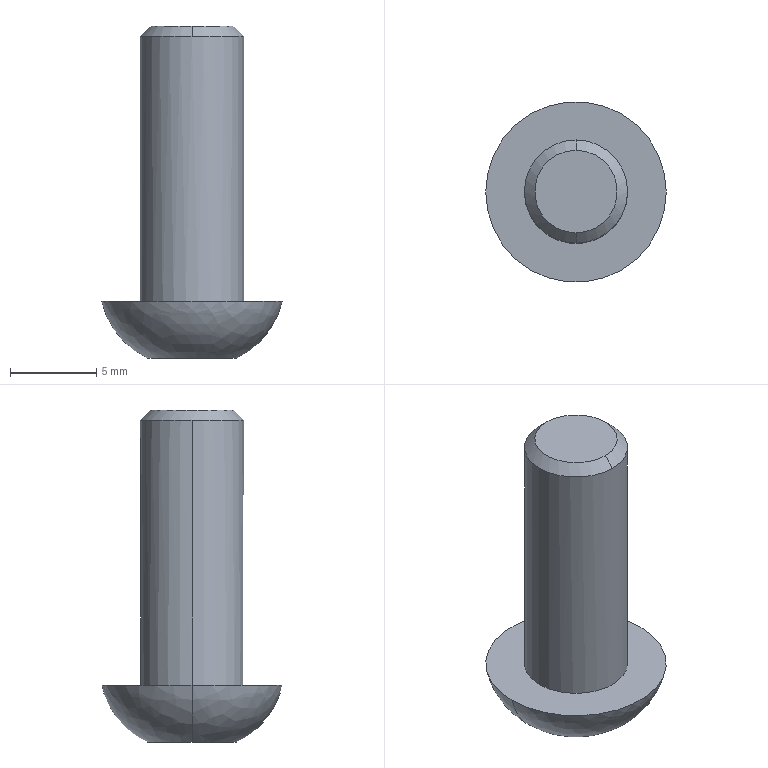Part | STEP file | LE-BYS-M6X16_PN_0013 | 1 solid | 23 faces | box 10.5 x 10.5 x 19.3 mm | volume 623.238 mm3 | plane 15 | cone 4 | spline 2 | cylinder 2 | commonest cylinder face diameters 6 x2
STEP:
#1=CARTESIAN_POINT('',(-2.6,0.,-3.3));
#2=VERTEX_POINT('',#1);
#3=CARTESIAN_POINT('',(2.6,0.,-3.3));
#4=VERTEX_POINT('',#3);
#5=CARTESIAN_POINT('',(0.,0.,-3.3));
#6=DIRECTION('',(0.,0.,1.));
#7=DIRECTION('',(-1.,0.,0.));
#8=AXIS2_PLACEMENT_3D('',#5,#6,#7);
#9=CIRCLE('',#8,2.6);
#10=EDGE_CURVE('',#2,#4,#9,.T.);
#11=ORIENTED_EDGE('',*,*,#10,.T.);
#12=CARTESIAN_POINT('',(5.25,0.,0.));
#13=VERTEX_POINT('',#12);
#14=CARTESIAN_POINT('',(0.5657,0.,1.048));
#15=DIRECTION('',(0.,-1.,0.));
#16=DIRECTION('',(1.,0.,0.));
#17=AXIS2_PLACEMENT_3D('',#14,#15,#16);
#18=CIRCLE('',#17,4.8);
#19=EDGE_CURVE('',#4,#13,#18,.T.);
#20=ORIENTED_EDGE('',*,*,#19,.T.);
#21=CARTESIAN_POINT('',(-5.25,0.,0.));
#22=VERTEX_POINT('',#21);
#23=CARTESIAN_POINT('',(0.,0.,0.));
#24=DIRECTION('',(0.,0.,1.));
#25=DIRECTION('',(-1.,0.,0.));
#26=AXIS2_PLACEMENT_3D('',#23,#24,#25);
#27=CIRCLE('',#26,5.25);
#28=EDGE_CURVE('',#22,#13,#27,.T.);
#29=ORIENTED_EDGE('',*,*,#28,.F.);
#30=CARTESIAN_POINT('',(-0.5657,0.,1.048));
#31=DIRECTION('',(0.,1.,0.));
#32=DIRECTION('',(-1.,0.,0.));
#33=AXIS2_PLACEMENT_3D('',#30,#31,#32);
#34=CIRCLE('',#33,4.8);
#35=EDGE_CURVE('',#2,#22,#34,.T.);
#36=ORIENTED_EDGE('',*,*,#35,.F.);
#37=EDGE_LOOP('',(#11,#20,#29,#36));
#38=FACE_OUTER_BOUND('',#37,.T.);
#39=CARTESIAN_POINT('',(2.6,0.,-3.3));
#40=CARTESIAN_POINT('',(2.6,-5.2,-3.3));
#41=CARTESIAN_POINT('',(-2.6,-5.2,-3.3));
#42=CARTESIAN_POINT('',(-2.6,0.,-3.3));
#43=CARTESIAN_POINT('',(3.971,0.,-2.658));
#44=CARTESIAN_POINT('',(3.971,-7.943,-2.658));
#45=CARTESIAN_POINT('',(-3.971,-7.943,-2.658));
#46=CARTESIAN_POINT('',(-3.971,0.,-2.658));
#47=CARTESIAN_POINT('',(4.92,0.,-1.478));
#48=CARTESIAN_POINT('',(4.92,-9.839,-1.478));
#49=CARTESIAN_POINT('',(-4.92,-9.839,-1.478));
#50=CARTESIAN_POINT('',(-4.92,0.,-1.478));
#51=CARTESIAN_POINT('',(5.25,0.,0.));
#52=CARTESIAN_POINT('',(5.25,-10.5,0.));
#53=CARTESIAN_POINT('',(-5.25,-10.5,0.));
#54=CARTESIAN_POINT('',(-5.25,0.,0.));
#55=(BOUNDED_SURFACE()B_SPLINE_SURFACE(3,3,((#39,#40,#41,#42),(#43,#44,#45,#46),(#47,#48,#49,#50),(#51,#52,#53,#54)),.UNSPECIFIED.,.F.,.F.,.T.)B_SPLINE_SURFACE_WITH_KNOTS((4,4),(4,4),(0.,1.),(0.,1.),.UNSPECIFIED.)GEOMETRIC_REPRESENTATION_ITEM()RATIONAL_B_SPLINE_SURFACE(((1.,0.3333,0.3333,1.),(0.9317,0.3106,0.3106,0.9317),(0.9317,0.3106,0.3106,0.9317),(1.,0.3333,0.3333,1.)))REPRESENTATION_ITEM('')SURFACE());
#56=ADVANCED_FACE('',(#38),#55,.T.);
#57=CARTESIAN_POINT('',(0.,3.,15.4));
#58=VERTEX_POINT('',#57);
#59=CARTESIAN_POINT('',(3.,0.,15.4));
#60=VERTEX_POINT('',#59);
#61=CARTESIAN_POINT('',(0.,0.,15.4));
#62=DIRECTION('',(0.,0.,-1.));
#63=DIRECTION('',(-1.,0.,0.));
#64=AXIS2_PLACEMENT_3D('',#61,#62,#63);
#65=CIRCLE('',#64,3.);
#66=EDGE_CURVE('',#58,#60,#65,.T.);
#67=ORIENTED_EDGE('',*,*,#66,.T.);
#68=CARTESIAN_POINT('',(3.,0.,0.));
#69=VERTEX_POINT('',#68);
#70=CARTESIAN_POINT('',(3.,0.,16.));
#71=DIRECTION('',(0.,0.,-1.));
#72=VECTOR('',#71,1000.);
#73=LINE('',#70,#72);
#74=EDGE_CURVE('',#60,#69,#73,.T.);
#75=ORIENTED_EDGE('',*,*,#74,.T.);
#76=CARTESIAN_POINT('',(-3.,0.,0.));
#77=VERTEX_POINT('',#76);
#78=CARTESIAN_POINT('',(0.,0.,0.));
#79=DIRECTION('',(0.,0.,1.));
#80=DIRECTION('',(-1.,0.,0.));
#81=AXIS2_PLACEMENT_3D('',#78,#79,#80);
#82=CIRCLE('',#81,3.);
#83=EDGE_CURVE('',#69,#77,#82,.T.);
#84=ORIENTED_EDGE('',*,*,#83,.T.);
#85=CARTESIAN_POINT('',(-3.,0.,15.4));
#86=VERTEX_POINT('',#85);
#87=CARTESIAN_POINT('',(-3.,0.,16.));
#88=DIRECTION('',(0.,0.,-1.));
#89=VECTOR('',#88,1000.);
#90=LINE('',#87,#89);
#91=EDGE_CURVE('',#86,#77,#90,.T.);
#92=ORIENTED_EDGE('',*,*,#91,.F.);
#93=CARTESIAN_POINT('',(0.,0.,15.4));
#94=DIRECTION('',(0.,0.,-1.));
#95=DIRECTION('',(-1.,0.,0.));
#96=AXIS2_PLACEMENT_3D('',#93,#94,#95);
#97=CIRCLE('',#96,3.);
#98=EDGE_CURVE('',#86,#58,#97,.T.);
#99=ORIENTED_EDGE('',*,*,#98,.T.);
#100=EDGE_LOOP('',(#67,#75,#84,#92,#99));
#101=FACE_OUTER_BOUND('',#100,.T.);
#102=CARTESIAN_POINT('',(0.,0.,16.));
#103=DIRECTION('',(0.,0.,-1.));
#104=DIRECTION('',(-1.,0.,0.));
#105=AXIS2_PLACEMENT_3D('',#102,#103,#104);
#106=CYLINDRICAL_SURFACE('',#105,3.);
#107=ADVANCED_FACE('',(#101),#106,.T.);
#108=CARTESIAN_POINT('',(0.,2.4,16.));
#109=VERTEX_POINT('',#108);
#110=CARTESIAN_POINT('',(0.,-2.4,16.));
#111=VERTEX_POINT('',#110);
#112=CARTESIAN_POINT('',(0.,0.,16.));
#113=DIRECTION('',(0.,0.,-1.));
#114=DIRECTION('',(0.,1.,0.));
#115=AXIS2_PLACEMENT_3D('',#112,#113,#114);
#116=CIRCLE('',#115,2.4);
#117=EDGE_CURVE('',#109,#111,#116,.T.);
#118=ORIENTED_EDGE('',*,*,#117,.T.);
#119=CARTESIAN_POINT('',(0.,-3.,15.4));
#120=VERTEX_POINT('',#119);
#121=CARTESIAN_POINT('',(0.,-3.,15.4));
#122=DIRECTION('',(0.,-0.7071,-0.7071));
#123=VECTOR('',#122,1000.);
#124=LINE('',#121,#123);
#125=EDGE_CURVE('',#111,#120,#124,.T.);
#126=ORIENTED_EDGE('',*,*,#125,.T.);
#127=CARTESIAN_POINT('',(0.,0.,15.4));
#128=DIRECTION('',(0.,0.,-1.));
#129=DIRECTION('',(-1.,0.,0.));
#130=AXIS2_PLACEMENT_3D('',#127,#128,#129);
#131=CIRCLE('',#130,3.);
#132=EDGE_CURVE('',#60,#120,#131,.T.);
#133=ORIENTED_EDGE('',*,*,#132,.F.);
#134=ORIENTED_EDGE('',*,*,#66,.F.);
#135=CARTESIAN_POINT('',(0.,3.,15.4));
#136=DIRECTION('',(0.,0.7071,-0.7071));
#137=VECTOR('',#136,1000.);
#138=LINE('',#135,#137);
#139=EDGE_CURVE('',#109,#58,#138,.T.);
#140=ORIENTED_EDGE('',*,*,#139,.F.);
#141=EDGE_LOOP('',(#118,#126,#133,#134,#140));
#142=FACE_OUTER_BOUND('',#141,.T.);
#143=CARTESIAN_POINT('',(0.,0.,15.4));
#144=DIRECTION('',(0.,0.,-1.));
#145=DIRECTION('',(0.,1.,0.));
#146=AXIS2_PLACEMENT_3D('',#143,#144,#145);
#147=CONICAL_SURFACE('',#146,3.,0.7854);
#148=ADVANCED_FACE('',(#142),#147,.T.);
#149=CARTESIAN_POINT('',(0.,0.,-0.4953));
#150=VERTEX_POINT('',#149);
#151=CARTESIAN_POINT('',(0.,2.,-1.65));
#152=VERTEX_POINT('',#151);
#153=CARTESIAN_POINT('',(0.,2.,-1.65));
#154=DIRECTION('',(0.,0.866,-0.5));
#155=VECTOR('',#154,1000.);
#156=LINE('',#153,#155);
#157=EDGE_CURVE('',#150,#152,#156,.T.);
#158=ORIENTED_EDGE('',*,*,#157,.F.);
#159=CARTESIAN_POINT('',(0.,-2.,-1.65));
#160=VERTEX_POINT('',#159);
#161=CARTESIAN_POINT('',(0.,-2.,-1.65));
#162=DIRECTION('',(0.,-0.866,-0.5));
#163=VECTOR('',#162,1000.);
#164=LINE('',#161,#163);
#165=EDGE_CURVE('',#150,#160,#164,.T.);
#166=ORIENTED_EDGE('',*,*,#165,.T.);
#167=CARTESIAN_POINT('',(-1.732,-1.,-1.65));
#168=VERTEX_POINT('',#167);
#169=CARTESIAN_POINT('',(0.,0.,-1.65));
#170=DIRECTION('',(0.,0.,1.));
#171=DIRECTION('',(0.,1.,0.));
#172=AXIS2_PLACEMENT_3D('',#169,#170,#171);
#173=CIRCLE('',#172,2.);
#174=EDGE_CURVE('',#168,#160,#173,.T.);
#175=ORIENTED_EDGE('',*,*,#174,.F.);
#176=CARTESIAN_POINT('',(-1.732,1.,-1.65));
#177=VERTEX_POINT('',#176);
#178=CARTESIAN_POINT('',(0.,0.,-1.65));
#179=DIRECTION('',(0.,0.,-1.));
#180=DIRECTION('',(0.,1.,0.));
#181=AXIS2_PLACEMENT_3D('',#178,#179,#180);
#182=CIRCLE('',#181,2.);
#183=EDGE_CURVE('',#168,#177,#182,.T.);
#184=ORIENTED_EDGE('',*,*,#183,.T.);
#185=CARTESIAN_POINT('',(0.,0.,-1.65));
#186=DIRECTION('',(0.,0.,1.));
#187=DIRECTION('',(0.,1.,0.));
#188=AXIS2_PLACEMENT_3D('',#185,#186,#187);
#189=CIRCLE('',#188,2.);
#190=EDGE_CURVE('',#152,#177,#189,.T.);
#191=ORIENTED_EDGE('',*,*,#190,.F.);
#192=EDGE_LOOP('',(#158,#166,#175,#184,#191));
#193=FACE_OUTER_BOUND('',#192,.T.);
#194=CARTESIAN_POINT('',(0.,0.,-1.65));
#195=DIRECTION('',(0.,0.,-1.));
#196=DIRECTION('',(0.,1.,0.));
#197=AXIS2_PLACEMENT_3D('',#194,#195,#196);
#198=CONICAL_SURFACE('',#197,2.,1.047);
#199=ADVANCED_FACE('',(#193),#198,.F.);
#200=ORIENTED_EDGE('',*,*,#74,.F.);
#201=ORIENTED_EDGE('',*,*,#132,.T.);
#202=CARTESIAN_POINT('',(0.,0.,15.4));
#203=DIRECTION('',(0.,0.,-1.));
#204=DIRECTION('',(-1.,0.,0.));
#205=AXIS2_PLACEMENT_3D('',#202,#203,#204);
#206=CIRCLE('',#205,3.);
#207=EDGE_CURVE('',#120,#86,#206,.T.);
#208=ORIENTED_EDGE('',*,*,#207,.T.);
#209=ORIENTED_EDGE('',*,*,#91,.T.);
#210=CARTESIAN_POINT('',(0.,0.,0.));
#211=DIRECTION('',(0.,0.,1.));
#212=DIRECTION('',(-1.,0.,0.));
#213=AXIS2_PLACEMENT_3D('',#210,#211,#212);
#214=CIRCLE('',#213,3.);
#215=EDGE_CURVE('',#77,#69,#214,.T.);
#216=ORIENTED_EDGE('',*,*,#215,.T.);
#217=EDGE_LOOP('',(#200,#201,#208,#209,#216));
#218=FACE_OUTER_BOUND('',#217,.T.);
#219=CARTESIAN_POINT('',(0.,0.,16.));
#220=DIRECTION('',(0.,0.,-1.));
#221=DIRECTION('',(-1.,0.,0.));
#222=AXIS2_PLACEMENT_3D('',#219,#220,#221);
#223=CYLINDRICAL_SURFACE('',#222,3.);
#224=ADVANCED_FACE('',(#218),#223,.T.);
#225=ORIENTED_EDGE('',*,*,#28,.T.);
#226=CARTESIAN_POINT('',(0.,0.,0.));
#227=DIRECTION('',(0.,0.,1.));
#228=DIRECTION('',(-1.,0.,0.));
#229=AXIS2_PLACEMENT_3D('',#226,#227,#228);
#230=CIRCLE('',#229,5.25);
#231=EDGE_CURVE('',#13,#22,#230,.T.);
#232=ORIENTED_EDGE('',*,*,#231,.T.);
#233=EDGE_LOOP('',(#225,#232));
#234=FACE_OUTER_BOUND('',#233,.T.);
#235=ORIENTED_EDGE('',*,*,#215,.F.);
#236=ORIENTED_EDGE('',*,*,#83,.F.);
#237=EDGE_LOOP('',(#235,#236));
#238=FACE_BOUND('',#237,.T.);
#239=CARTESIAN_POINT('',(0.,0.,0.));
#240=DIRECTION('',(0.,0.,1.));
#241=DIRECTION('',(1.,0.,0.));
#242=AXIS2_PLACEMENT_3D('',#239,#240,#241);
#243=PLANE('',#242);
#244=ADVANCED_FACE('',(#234,#238),#243,.T.);
#245=ORIENTED_EDGE('',*,*,#125,.F.);
#246=CARTESIAN_POINT('',(0.,0.,16.));
#247=DIRECTION('',(0.,0.,-1.));
#248=DIRECTION('',(0.,1.,0.));
#249=AXIS2_PLACEMENT_3D('',#246,#247,#248);
#250=CIRCLE('',#249,2.4);
#251=EDGE_CURVE('',#111,#109,#250,.T.);
#252=ORIENTED_EDGE('',*,*,#251,.T.);
#253=ORIENTED_EDGE('',*,*,#139,.T.);
#254=ORIENTED_EDGE('',*,*,#98,.F.);
#255=ORIENTED_EDGE('',*,*,#207,.F.);
#256=EDGE_LOOP('',(#245,#252,#253,#254,#255));
#257=FACE_OUTER_BOUND('',#256,.T.);
#258=CARTESIAN_POINT('',(0.,0.,15.4));
#259=DIRECTION('',(0.,0.,-1.));
#260=DIRECTION('',(0.,1.,0.));
#261=AXIS2_PLACEMENT_3D('',#258,#259,#260);
#262=CONICAL_SURFACE('',#261,3.,0.7854);
#263=ADVANCED_FACE('',(#257),#262,.T.);
#264=ORIENTED_EDGE('',*,*,#19,.F.);
#265=CARTESIAN_POINT('',(0.,0.,-3.3));
#266=DIRECTION('',(0.,0.,1.));
#267=DIRECTION('',(-1.,0.,0.));
#268=AXIS2_PLACEMENT_3D('',#265,#266,#267);
#269=CIRCLE('',#268,2.6);
#270=EDGE_CURVE('',#4,#2,#269,.T.);
#271=ORIENTED_EDGE('',*,*,#270,.T.);
#272=ORIENTED_EDGE('',*,*,#35,.T.);
#273=ORIENTED_EDGE('',*,*,#231,.F.);
#274=EDGE_LOOP('',(#264,#271,#272,#273));
#275=FACE_OUTER_BOUND('',#274,.T.);
#276=CARTESIAN_POINT('',(-2.6,0.,-3.3));
#277=CARTESIAN_POINT('',(-2.6,5.2,-3.3));
#278=CARTESIAN_POINT('',(2.6,5.2,-3.3));
#279=CARTESIAN_POINT('',(2.6,0.,-3.3));
#280=CARTESIAN_POINT('',(-3.971,0.,-2.658));
#281=CARTESIAN_POINT('',(-3.971,7.943,-2.658));
#282=CARTESIAN_POINT('',(3.971,7.943,-2.658));
#283=CARTESIAN_POINT('',(3.971,0.,-2.658));
#284=CARTESIAN_POINT('',(-4.92,0.,-1.478));
#285=CARTESIAN_POINT('',(-4.92,9.839,-1.478));
#286=CARTESIAN_POINT('',(4.92,9.839,-1.478));
#287=CARTESIAN_POINT('',(4.92,0.,-1.478));
#288=CARTESIAN_POINT('',(-5.25,0.,0.));
#289=CARTESIAN_POINT('',(-5.25,10.5,0.));
#290=CARTESIAN_POINT('',(5.25,10.5,0.));
#291=CARTESIAN_POINT('',(5.25,0.,0.));
#292=(BOUNDED_SURFACE()B_SPLINE_SURFACE(3,3,((#276,#277,#278,#279),(#280,#281,#282,#283),(#284,#285,#286,#287),(#288,#289,#290,#291)),.UNSPECIFIED.,.F.,.F.,.F.)B_SPLINE_SURFACE_WITH_KNOTS((4,4),(4,4),(0.,1.),(0.,1.),.UNSPECIFIED.)GEOMETRIC_REPRESENTATION_ITEM()RATIONAL_B_SPLINE_SURFACE(((1.,0.3333,0.3333,1.),(0.9317,0.3106,0.3106,0.9317),(0.9317,0.3106,0.3106,0.9317),(1.,0.3333,0.3333,1.)))REPRESENTATION_ITEM('')SURFACE());
#293=ADVANCED_FACE('',(#275),#292,.T.);
#294=ORIENTED_EDGE('',*,*,#117,.F.);
#295=ORIENTED_EDGE('',*,*,#251,.F.);
#296=EDGE_LOOP('',(#294,#295));
#297=FACE_OUTER_BOUND('',#296,.T.);
#298=CARTESIAN_POINT('',(0.,0.,16.));
#299=DIRECTION('',(0.,0.,-1.));
#300=DIRECTION('',(-1.,0.,0.));
#301=AXIS2_PLACEMENT_3D('',#298,#299,#300);
#302=PLANE('',#301);
#303=ADVANCED_FACE('',(#297),#302,.F.);
#304=CARTESIAN_POINT('',(-1.155,2.,-3.3));
#305=VERTEX_POINT('',#304);
#306=CARTESIAN_POINT('',(1.155,2.,-3.3));
#307=VERTEX_POINT('',#306);
#308=CARTESIAN_POINT('',(0.,2.,-3.3));
#309=DIRECTION('',(1.,0.,0.));
#310=VECTOR('',#309,1000.);
#311=LINE('',#308,#310);
#312=EDGE_CURVE('',#305,#307,#311,.T.);
#313=ORIENTED_EDGE('',*,*,#312,.F.);
#314=CARTESIAN_POINT('',(-2.309,0.,-3.3));
#315=VERTEX_POINT('',#314);
#316=CARTESIAN_POINT('',(-2.309,0.,-3.3));
#317=DIRECTION('',(0.5,0.866,0.));
#318=VECTOR('',#317,1000.);
#319=LINE('',#316,#318);
#320=EDGE_CURVE('',#315,#305,#319,.T.);
#321=ORIENTED_EDGE('',*,*,#320,.F.);
#322=CARTESIAN_POINT('',(-1.155,-2.,-3.3));
#323=VERTEX_POINT('',#322);
#324=CARTESIAN_POINT('',(-1.155,-2.,-3.3));
#325=DIRECTION('',(-0.5,0.866,0.));
#326=VECTOR('',#325,1000.);
#327=LINE('',#324,#326);
#328=EDGE_CURVE('',#323,#315,#327,.T.);
#329=ORIENTED_EDGE('',*,*,#328,.F.);
#330=CARTESIAN_POINT('',(1.155,-2.,-3.3));
#331=VERTEX_POINT('',#330);
#332=CARTESIAN_POINT('',(0.,-2.,-3.3));
#333=DIRECTION('',(-1.,0.,0.));
#334=VECTOR('',#333,1000.);
#335=LINE('',#332,#334);
#336=EDGE_CURVE('',#331,#323,#335,.T.);
#337=ORIENTED_EDGE('',*,*,#336,.F.);
#338=CARTESIAN_POINT('',(2.309,0.,-3.3));
#339=VERTEX_POINT('',#338);
#340=CARTESIAN_POINT('',(2.309,0.,-3.3));
#341=DIRECTION('',(-0.5,-0.866,0.));
#342=VECTOR('',#341,1000.);
#343=LINE('',#340,#342);
#344=EDGE_CURVE('',#339,#331,#343,.T.);
#345=ORIENTED_EDGE('',*,*,#344,.F.);
#346=CARTESIAN_POINT('',(1.155,2.,-3.3));
#347=DIRECTION('',(0.5,-0.866,0.));
#348=VECTOR('',#347,1000.);
#349=LINE('',#346,#348);
#350=EDGE_CURVE('',#307,#339,#349,.T.);
#351=ORIENTED_EDGE('',*,*,#350,.F.);
#352=EDGE_LOOP('',(#313,#321,#329,#337,#345,#351));
#353=FACE_BOUND('',#352,.T.);
#354=ORIENTED_EDGE('',*,*,#10,.F.);
#355=ORIENTED_EDGE('',*,*,#270,.F.);
#356=EDGE_LOOP('',(#354,#355));
#357=FACE_OUTER_BOUND('',#356,.T.);
#358=CARTESIAN_POINT('',(0.,0.,-3.3));
#359=DIRECTION('',(0.,0.,1.));
#360=DIRECTION('',(1.,0.,0.));
#361=AXIS2_PLACEMENT_3D('',#358,#359,#360);
#362=PLANE('',#361);
#363=ADVANCED_FACE('',(#353,#357),#362,.F.);
#364=CARTESIAN_POINT('',(1.732,1.,-1.65));
#365=VERTEX_POINT('',#364);
#366=CARTESIAN_POINT('',(1.155,2.,-1.65));
#367=VERTEX_POINT('',#366);
#368=CARTESIAN_POINT('',(2.309,0.,-1.65));
#369=DIRECTION('',(-0.5,0.866,0.));
#370=VECTOR('',#369,1000.);
#371=LINE('',#368,#370);
#372=EDGE_CURVE('',#365,#367,#371,.T.);
#373=ORIENTED_EDGE('',*,*,#372,.T.);
#374=CARTESIAN_POINT('',(1.155,2.,-1.65));
#375=DIRECTION('',(0.,0.,-1.));
#376=VECTOR('',#375,1000.);
#377=LINE('',#374,#376);
#378=EDGE_CURVE('',#367,#307,#377,.T.);
#379=ORIENTED_EDGE('',*,*,#378,.T.);
#380=ORIENTED_EDGE('',*,*,#350,.T.);
#381=CARTESIAN_POINT('',(2.309,0.,-1.65));
#382=VERTEX_POINT('',#381);
#383=CARTESIAN_POINT('',(2.309,0.,-1.65));
#384=DIRECTION('',(0.,0.,1.));
#385=VECTOR('',#384,1000.);
#386=LINE('',#383,#385);
#387=EDGE_CURVE('',#339,#382,#386,.T.);
#388=ORIENTED_EDGE('',*,*,#387,.T.);
#389=CARTESIAN_POINT('',(2.309,0.,-1.65));
#390=DIRECTION('',(-0.5,0.866,0.));
#391=VECTOR('',#390,1000.);
#392=LINE('',#389,#391);
#393=EDGE_CURVE('',#382,#365,#392,.T.);
#394=ORIENTED_EDGE('',*,*,#393,.T.);
#395=EDGE_LOOP('',(#373,#379,#380,#388,#394));
#396=FACE_OUTER_BOUND('',#395,.T.);
#397=CARTESIAN_POINT('',(2.309,0.,-1.65));
#398=DIRECTION('',(-0.866,-0.5,0.));
#399=DIRECTION('',(0.5,-0.866,0.));
#400=AXIS2_PLACEMENT_3D('',#397,#398,#399);
#401=PLANE('',#400);
#402=ADVANCED_FACE('',(#396),#401,.T.);
#403=CARTESIAN_POINT('',(-1.155,2.,-1.65));
#404=VERTEX_POINT('',#403);
#405=CARTESIAN_POINT('',(0.,2.,-1.65));
#406=DIRECTION('',(-1.,0.,0.));
#407=VECTOR('',#406,1000.);
#408=LINE('',#405,#407);
#409=EDGE_CURVE('',#152,#404,#408,.T.);
#410=ORIENTED_EDGE('',*,*,#409,.T.);
#411=CARTESIAN_POINT('',(-1.155,2.,-1.65));
#412=DIRECTION('',(0.,0.,-1.));
#413=VECTOR('',#412,1000.);
#414=LINE('',#411,#413);
#415=EDGE_CURVE('',#404,#305,#414,.T.);
#416=ORIENTED_EDGE('',*,*,#415,.T.);
#417=ORIENTED_EDGE('',*,*,#312,.T.);
#418=ORIENTED_EDGE('',*,*,#378,.F.);
#419=CARTESIAN_POINT('',(1.155,2.,-1.65));
#420=DIRECTION('',(-1.,0.,0.));
#421=VECTOR('',#420,1000.);
#422=LINE('',#419,#421);
#423=EDGE_CURVE('',#367,#152,#422,.T.);
#424=ORIENTED_EDGE('',*,*,#423,.T.);
#425=EDGE_LOOP('',(#410,#416,#417,#418,#424));
#426=FACE_OUTER_BOUND('',#425,.T.);
#427=CARTESIAN_POINT('',(1.155,2.,-1.65));
#428=DIRECTION('',(0.,-1.,0.));
#429=DIRECTION('',(0.,0.,-1.));
#430=AXIS2_PLACEMENT_3D('',#427,#428,#429);
#431=PLANE('',#430);
#432=ADVANCED_FACE('',(#426),#431,.T.);
#433=CARTESIAN_POINT('',(-2.309,0.,-1.65));
#434=VERTEX_POINT('',#433);
#435=CARTESIAN_POINT('',(-1.155,2.,-1.65));
#436=DIRECTION('',(-0.5,-0.866,0.));
#437=VECTOR('',#436,1000.);
#438=LINE('',#435,#437);
#439=EDGE_CURVE('',#177,#434,#438,.T.);
#440=ORIENTED_EDGE('',*,*,#439,.T.);
#441=CARTESIAN_POINT('',(-2.309,0.,-1.65));
#442=DIRECTION('',(0.,0.,-1.));
#443=VECTOR('',#442,1000.);
#444=LINE('',#441,#443);
#445=EDGE_CURVE('',#434,#315,#444,.T.);
#446=ORIENTED_EDGE('',*,*,#445,.T.);
#447=ORIENTED_EDGE('',*,*,#320,.T.);
#448=ORIENTED_EDGE('',*,*,#415,.F.);
#449=CARTESIAN_POINT('',(-1.155,2.,-1.65));
#450=DIRECTION('',(-0.5,-0.866,0.));
#451=VECTOR('',#450,1000.);
#452=LINE('',#449,#451);
#453=EDGE_CURVE('',#404,#177,#452,.T.);
#454=ORIENTED_EDGE('',*,*,#453,.T.);
#455=EDGE_LOOP('',(#440,#446,#447,#448,#454));
#456=FACE_OUTER_BOUND('',#455,.T.);
#457=CARTESIAN_POINT('',(-1.155,2.,-1.65));
#458=DIRECTION('',(0.866,-0.5,0.));
#459=DIRECTION('',(0.5,0.866,0.));
#460=AXIS2_PLACEMENT_3D('',#457,#458,#459);
#461=PLANE('',#460);
#462=ADVANCED_FACE('',(#456),#461,.T.);
#463=CARTESIAN_POINT('',(-1.155,-2.,-1.65));
#464=VERTEX_POINT('',#463);
#465=CARTESIAN_POINT('',(-1.732,-1.,-1.65));
#466=DIRECTION('',(0.5,-0.866,0.));
#467=VECTOR('',#466,1000.);
#468=LINE('',#465,#467);
#469=EDGE_CURVE('',#168,#464,#468,.T.);
#470=ORIENTED_EDGE('',*,*,#469,.T.);
#471=CARTESIAN_POINT('',(-1.155,-2.,-1.65));
#472=DIRECTION('',(0.,0.,-1.));
#473=VECTOR('',#472,1000.);
#474=LINE('',#471,#473);
#475=EDGE_CURVE('',#464,#323,#474,.T.);
#476=ORIENTED_EDGE('',*,*,#475,.T.);
#477=ORIENTED_EDGE('',*,*,#328,.T.);
#478=ORIENTED_EDGE('',*,*,#445,.F.);
#479=CARTESIAN_POINT('',(-2.309,0.,-1.65));
#480=DIRECTION('',(0.5,-0.866,0.));
#481=VECTOR('',#480,1000.);
#482=LINE('',#479,#481);
#483=EDGE_CURVE('',#434,#168,#482,.T.);
#484=ORIENTED_EDGE('',*,*,#483,.T.);
#485=EDGE_LOOP('',(#470,#476,#477,#478,#484));
#486=FACE_OUTER_BOUND('',#485,.T.);
#487=CARTESIAN_POINT('',(-2.309,0.,-1.65));
#488=DIRECTION('',(0.866,0.5,0.));
#489=DIRECTION('',(-0.5,0.866,0.));
#490=AXIS2_PLACEMENT_3D('',#487,#488,#489);
#491=PLANE('',#490);
#492=ADVANCED_FACE('',(#486),#491,.T.);
#493=CARTESIAN_POINT('',(1.155,-2.,-1.65));
#494=VERTEX_POINT('',#493);
#495=CARTESIAN_POINT('',(0.,-2.,-1.65));
#496=DIRECTION('',(1.,0.,0.));
#497=VECTOR('',#496,1000.);
#498=LINE('',#495,#497);
#499=EDGE_CURVE('',#160,#494,#498,.T.);
#500=ORIENTED_EDGE('',*,*,#499,.T.);
#501=CARTESIAN_POINT('',(1.155,-2.,-1.65));
#502=DIRECTION('',(0.,0.,-1.));
#503=VECTOR('',#502,1000.);
#504=LINE('',#501,#503);
#505=EDGE_CURVE('',#494,#331,#504,.T.);
#506=ORIENTED_EDGE('',*,*,#505,.T.);
#507=ORIENTED_EDGE('',*,*,#336,.T.);
#508=ORIENTED_EDGE('',*,*,#475,.F.);
#509=CARTESIAN_POINT('',(0.,-2.,-1.65));
#510=DIRECTION('',(1.,0.,0.));
#511=VECTOR('',#510,1000.);
#512=LINE('',#509,#511);
#513=EDGE_CURVE('',#464,#160,#512,.T.);
#514=ORIENTED_EDGE('',*,*,#513,.T.);
#515=EDGE_LOOP('',(#500,#506,#507,#508,#514));
#516=FACE_OUTER_BOUND('',#515,.T.);
#517=CARTESIAN_POINT('',(-1.155,-2.,-1.65));
#518=DIRECTION('',(0.,1.,0.));
#519=DIRECTION('',(0.,0.,1.));
#520=AXIS2_PLACEMENT_3D('',#517,#518,#519);
#521=PLANE('',#520);
#522=ADVANCED_FACE('',(#516),#521,.T.);
#523=CARTESIAN_POINT('',(1.732,-1.,-1.65));
#524=VERTEX_POINT('',#523);
#525=CARTESIAN_POINT('',(1.155,-2.,-1.65));
#526=DIRECTION('',(0.5,0.866,0.));
#527=VECTOR('',#526,1000.);
#528=LINE('',#525,#527);
#529=EDGE_CURVE('',#524,#382,#528,.T.);
#530=ORIENTED_EDGE('',*,*,#529,.T.);
#531=ORIENTED_EDGE('',*,*,#387,.F.);
#532=ORIENTED_EDGE('',*,*,#344,.T.);
#533=ORIENTED_EDGE('',*,*,#505,.F.);
#534=CARTESIAN_POINT('',(1.155,-2.,-1.65));
#535=DIRECTION('',(0.5,0.866,0.));
#536=VECTOR('',#535,1000.);
#537=LINE('',#534,#536);
#538=EDGE_CURVE('',#494,#524,#537,.T.);
#539=ORIENTED_EDGE('',*,*,#538,.T.);
#540=EDGE_LOOP('',(#530,#531,#532,#533,#539));
#541=FACE_OUTER_BOUND('',#540,.T.);
#542=CARTESIAN_POINT('',(1.155,-2.,-1.65));
#543=DIRECTION('',(-0.866,0.5,0.));
#544=DIRECTION('',(-0.5,-0.866,0.));
#545=AXIS2_PLACEMENT_3D('',#542,#543,#544);
#546=PLANE('',#545);
#547=ADVANCED_FACE('',(#541),#546,.T.);
#548=CARTESIAN_POINT('',(0.,0.,-1.65));
#549=DIRECTION('',(0.,0.,-1.));
#550=DIRECTION('',(0.,1.,0.));
#551=AXIS2_PLACEMENT_3D('',#548,#549,#550);
#552=CIRCLE('',#551,2.);
#553=EDGE_CURVE('',#152,#365,#552,.T.);
#554=ORIENTED_EDGE('',*,*,#553,.F.);
#555=ORIENTED_EDGE('',*,*,#423,.F.);
#556=ORIENTED_EDGE('',*,*,#372,.F.);
#557=EDGE_LOOP('',(#554,#555,#556));
#558=FACE_OUTER_BOUND('',#557,.T.);
#559=CARTESIAN_POINT('',(0.,0.,-1.65));
#560=DIRECTION('',(0.,0.,1.));
#561=DIRECTION('',(1.,0.,0.));
#562=AXIS2_PLACEMENT_3D('',#559,#560,#561);
#563=PLANE('',#562);
#564=ADVANCED_FACE('',(#558),#563,.F.);
#565=ORIENTED_EDGE('',*,*,#529,.F.);
#566=CARTESIAN_POINT('',(0.,0.,-1.65));
#567=DIRECTION('',(0.,0.,-1.));
#568=DIRECTION('',(0.,1.,0.));
#569=AXIS2_PLACEMENT_3D('',#566,#567,#568);
#570=CIRCLE('',#569,2.);
#571=EDGE_CURVE('',#365,#524,#570,.T.);
#572=ORIENTED_EDGE('',*,*,#571,.F.);
#573=ORIENTED_EDGE('',*,*,#393,.F.);
#574=EDGE_LOOP('',(#565,#572,#573));
#575=FACE_OUTER_BOUND('',#574,.T.);
#576=CARTESIAN_POINT('',(0.,0.,-1.65));
#577=DIRECTION('',(0.,0.,1.));
#578=DIRECTION('',(1.,0.,0.));
#579=AXIS2_PLACEMENT_3D('',#576,#577,#578);
#580=PLANE('',#579);
#581=ADVANCED_FACE('',(#575),#580,.F.);
#582=ORIENTED_EDGE('',*,*,#183,.F.);
#583=ORIENTED_EDGE('',*,*,#483,.F.);
#584=ORIENTED_EDGE('',*,*,#439,.F.);
#585=EDGE_LOOP('',(#582,#583,#584));
#586=FACE_OUTER_BOUND('',#585,.T.);
#587=CARTESIAN_POINT('',(0.,0.,-1.65));
#588=DIRECTION('',(0.,0.,1.));
#589=DIRECTION('',(1.,0.,0.));
#590=AXIS2_PLACEMENT_3D('',#587,#588,#589);
#591=PLANE('',#590);
#592=ADVANCED_FACE('',(#586),#591,.F.);
#593=ORIENTED_EDGE('',*,*,#165,.F.);
#594=ORIENTED_EDGE('',*,*,#157,.T.);
#595=ORIENTED_EDGE('',*,*,#553,.T.);
#596=ORIENTED_EDGE('',*,*,#571,.T.);
#597=CARTESIAN_POINT('',(0.,0.,-1.65));
#598=DIRECTION('',(0.,0.,1.));
#599=DIRECTION('',(0.,1.,0.));
#600=AXIS2_PLACEMENT_3D('',#597,#598,#599);
#601=CIRCLE('',#600,2.);
#602=EDGE_CURVE('',#160,#524,#601,.T.);
#603=ORIENTED_EDGE('',*,*,#602,.F.);
#604=EDGE_LOOP('',(#593,#594,#595,#596,#603));
#605=FACE_OUTER_BOUND('',#604,.T.);
#606=CARTESIAN_POINT('',(0.,0.,-1.65));
#607=DIRECTION('',(0.,0.,-1.));
#608=DIRECTION('',(0.,1.,0.));
#609=AXIS2_PLACEMENT_3D('',#606,#607,#608);
#610=CONICAL_SURFACE('',#609,2.,1.047);
#611=ADVANCED_FACE('',(#605),#610,.F.);
#612=ORIENTED_EDGE('',*,*,#190,.T.);
#613=ORIENTED_EDGE('',*,*,#453,.F.);
#614=ORIENTED_EDGE('',*,*,#409,.F.);
#615=EDGE_LOOP('',(#612,#613,#614));
#616=FACE_OUTER_BOUND('',#615,.T.);
#617=CARTESIAN_POINT('',(0.,0.,-1.65));
#618=DIRECTION('',(0.,0.,1.));
#619=DIRECTION('',(1.,0.,0.));
#620=AXIS2_PLACEMENT_3D('',#617,#618,#619);
#621=PLANE('',#620);
#622=ADVANCED_FACE('',(#616),#621,.F.);
#623=ORIENTED_EDGE('',*,*,#602,.T.);
#624=ORIENTED_EDGE('',*,*,#538,.F.);
#625=ORIENTED_EDGE('',*,*,#499,.F.);
#626=EDGE_LOOP('',(#623,#624,#625));
#627=FACE_OUTER_BOUND('',#626,.T.);
#628=CARTESIAN_POINT('',(0.,0.,-1.65));
#629=DIRECTION('',(0.,0.,1.));
#630=DIRECTION('',(1.,0.,0.));
#631=AXIS2_PLACEMENT_3D('',#628,#629,#630);
#632=PLANE('',#631);
#633=ADVANCED_FACE('',(#627),#632,.F.);
#634=ORIENTED_EDGE('',*,*,#174,.T.);
#635=ORIENTED_EDGE('',*,*,#513,.F.);
#636=ORIENTED_EDGE('',*,*,#469,.F.);
#637=EDGE_LOOP('',(#634,#635,#636));
#638=FACE_OUTER_BOUND('',#637,.T.);
#639=CARTESIAN_POINT('',(0.,0.,-1.65));
#640=DIRECTION('',(0.,0.,1.));
#641=DIRECTION('',(1.,0.,0.));
#642=AXIS2_PLACEMENT_3D('',#639,#640,#641);
#643=PLANE('',#642);
#644=ADVANCED_FACE('',(#638),#643,.F.);
#645=CLOSED_SHELL('',(#56,#107,#148,#199,#224,#244,#263,#293,#303,#363,#402,#432,#462,#492,#522,#547,#564,#581,#592,#611,#622,#633,#644));
#646=MANIFOLD_SOLID_BREP('',#645);
#647=CARTESIAN_POINT('',(0.,0.,0.));
#648=DIRECTION('',(0.,0.,1.));
#649=DIRECTION('',(1.,0.,0.));
#650=AXIS2_PLACEMENT_3D('',#647,#648,#649);
#651=(LENGTH_UNIT()NAMED_UNIT(*)SI_UNIT(.MILLI.,.METRE.));
#652=UNCERTAINTY_MEASURE_WITH_UNIT(LENGTH_MEASURE(0.00001),#651,'','');
#653=(NAMED_UNIT(*)PLANE_ANGLE_UNIT()SI_UNIT($,.RADIAN.));
#654=(NAMED_UNIT(*)SI_UNIT($,.STERADIAN.)SOLID_ANGLE_UNIT());
#655=(GEOMETRIC_REPRESENTATION_CONTEXT(3)GLOBAL_UNCERTAINTY_ASSIGNED_CONTEXT((#652))GLOBAL_UNIT_ASSIGNED_CONTEXT((#651,#653,#654))REPRESENTATION_CONTEXT('',''));
#656=ADVANCED_BREP_SHAPE_REPRESENTATION('',(#646,#650),#655);